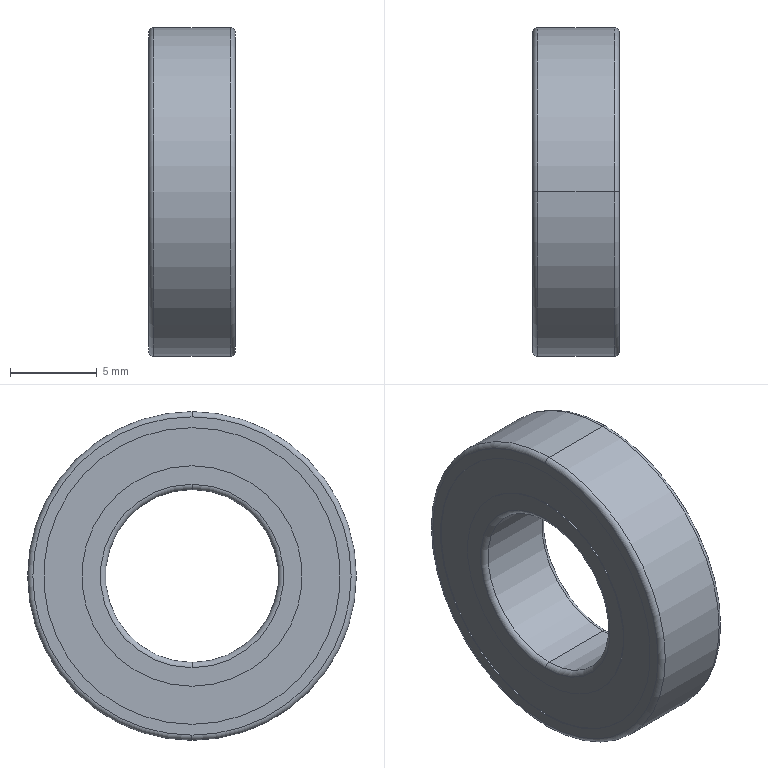Part | STEP file | 11-B6800ZZ11_B6800ZZ | 1 solid | 26 faces | box 5 x 19 x 19 mm | volume 1010 mm3 | cylinder 12 | torus 8 | plane 6 | commonest cylinder face diameters 12.74 x4 17.15 x4 10 x2 19 x2
STEP:
#1=CARTESIAN_POINT('',(4.7,0.,9.5));
#2=VERTEX_POINT('',#1);
#3=CARTESIAN_POINT('',(4.7,0.,-9.5));
#4=VERTEX_POINT('',#3);
#5=CARTESIAN_POINT('',(4.7,0.,0.));
#6=DIRECTION('',(-1.,0.,0.));
#7=DIRECTION('',(0.,0.,1.));
#8=AXIS2_PLACEMENT_3D('',#5,#6,#7);
#9=CIRCLE('',#8,9.5);
#10=EDGE_CURVE('',#2,#4,#9,.T.);
#11=ORIENTED_EDGE('',*,*,#10,.T.);
#12=CARTESIAN_POINT('',(0.3,0.,-9.5));
#13=VERTEX_POINT('',#12);
#14=CARTESIAN_POINT('',(5.,0.,-9.5));
#15=DIRECTION('',(-1.,0.,0.));
#16=VECTOR('',#15,1000.);
#17=LINE('',#14,#16);
#18=EDGE_CURVE('',#4,#13,#17,.T.);
#19=ORIENTED_EDGE('',*,*,#18,.T.);
#20=CARTESIAN_POINT('',(0.3,0.,9.5));
#21=VERTEX_POINT('',#20);
#22=CARTESIAN_POINT('',(0.3,0.,0.));
#23=DIRECTION('',(-1.,0.,0.));
#24=DIRECTION('',(0.,0.,1.));
#25=AXIS2_PLACEMENT_3D('',#22,#23,#24);
#26=CIRCLE('',#25,9.5);
#27=EDGE_CURVE('',#21,#13,#26,.T.);
#28=ORIENTED_EDGE('',*,*,#27,.F.);
#29=CARTESIAN_POINT('',(5.,0.,9.5));
#30=DIRECTION('',(-1.,0.,0.));
#31=VECTOR('',#30,1000.);
#32=LINE('',#29,#31);
#33=EDGE_CURVE('',#2,#21,#32,.T.);
#34=ORIENTED_EDGE('',*,*,#33,.F.);
#35=EDGE_LOOP('',(#11,#19,#28,#34));
#36=FACE_OUTER_BOUND('',#35,.T.);
#37=CARTESIAN_POINT('',(5.,0.,0.));
#38=DIRECTION('',(-1.,0.,0.));
#39=DIRECTION('',(0.,0.,1.));
#40=AXIS2_PLACEMENT_3D('',#37,#38,#39);
#41=CYLINDRICAL_SURFACE('',#40,9.5);
#42=ADVANCED_FACE('',(#36),#41,.T.);
#43=CARTESIAN_POINT('',(5.,0.,9.2));
#44=VERTEX_POINT('',#43);
#45=CARTESIAN_POINT('',(5.,0.,-9.2));
#46=VERTEX_POINT('',#45);
#47=CARTESIAN_POINT('',(5.,0.,0.));
#48=DIRECTION('',(-1.,0.,0.));
#49=DIRECTION('',(0.,0.,1.));
#50=AXIS2_PLACEMENT_3D('',#47,#48,#49);
#51=CIRCLE('',#50,9.2);
#52=EDGE_CURVE('',#44,#46,#51,.T.);
#53=ORIENTED_EDGE('',*,*,#52,.T.);
#54=CARTESIAN_POINT('',(4.7,0.,-9.2));
#55=DIRECTION('',(0.,1.,0.));
#56=DIRECTION('',(0.,0.,1.));
#57=AXIS2_PLACEMENT_3D('',#54,#55,#56);
#58=CIRCLE('',#57,0.3);
#59=EDGE_CURVE('',#46,#4,#58,.T.);
#60=ORIENTED_EDGE('',*,*,#59,.T.);
#61=ORIENTED_EDGE('',*,*,#10,.F.);
#62=CARTESIAN_POINT('',(4.7,0.,9.2));
#63=DIRECTION('',(0.,-1.,0.));
#64=DIRECTION('',(0.,0.,-1.));
#65=AXIS2_PLACEMENT_3D('',#62,#63,#64);
#66=CIRCLE('',#65,0.3);
#67=EDGE_CURVE('',#44,#2,#66,.T.);
#68=ORIENTED_EDGE('',*,*,#67,.F.);
#69=EDGE_LOOP('',(#53,#60,#61,#68));
#70=FACE_OUTER_BOUND('',#69,.T.);
#71=CARTESIAN_POINT('',(4.7,0.,0.));
#72=DIRECTION('',(-1.,0.,0.));
#73=DIRECTION('',(0.,0.,1.));
#74=AXIS2_PLACEMENT_3D('',#71,#72,#73);
#75=TOROIDAL_SURFACE('',#74,9.2,0.3);
#76=ADVANCED_FACE('',(#70),#75,.T.);
#77=CARTESIAN_POINT('',(5.,0.,-8.575));
#78=VERTEX_POINT('',#77);
#79=CARTESIAN_POINT('',(5.,0.,8.575));
#80=VERTEX_POINT('',#79);
#81=CARTESIAN_POINT('',(5.,0.,0.));
#82=DIRECTION('',(-1.,0.,0.));
#83=DIRECTION('',(0.,0.,1.));
#84=AXIS2_PLACEMENT_3D('',#81,#82,#83);
#85=CIRCLE('',#84,8.575);
#86=EDGE_CURVE('',#78,#80,#85,.T.);
#87=ORIENTED_EDGE('',*,*,#86,.F.);
#88=CARTESIAN_POINT('',(4.942,0.,-8.575));
#89=VERTEX_POINT('',#88);
#90=CARTESIAN_POINT('',(5.,0.,-8.575));
#91=DIRECTION('',(-1.,0.,0.));
#92=VECTOR('',#91,1000.);
#93=LINE('',#90,#92);
#94=EDGE_CURVE('',#78,#89,#93,.T.);
#95=ORIENTED_EDGE('',*,*,#94,.T.);
#96=CARTESIAN_POINT('',(4.942,0.,8.575));
#97=VERTEX_POINT('',#96);
#98=CARTESIAN_POINT('',(4.942,0.,0.));
#99=DIRECTION('',(-1.,0.,0.));
#100=DIRECTION('',(0.,0.,1.));
#101=AXIS2_PLACEMENT_3D('',#98,#99,#100);
#102=CIRCLE('',#101,8.575);
#103=EDGE_CURVE('',#89,#97,#102,.T.);
#104=ORIENTED_EDGE('',*,*,#103,.T.);
#105=CARTESIAN_POINT('',(5.,0.,8.575));
#106=DIRECTION('',(-1.,0.,0.));
#107=VECTOR('',#106,1000.);
#108=LINE('',#105,#107);
#109=EDGE_CURVE('',#80,#97,#108,.T.);
#110=ORIENTED_EDGE('',*,*,#109,.F.);
#111=EDGE_LOOP('',(#87,#95,#104,#110));
#112=FACE_OUTER_BOUND('',#111,.T.);
#113=CARTESIAN_POINT('',(5.,0.,0.));
#114=DIRECTION('',(-1.,0.,0.));
#115=DIRECTION('',(0.,0.,1.));
#116=AXIS2_PLACEMENT_3D('',#113,#114,#115);
#117=CYLINDRICAL_SURFACE('',#116,8.575);
#118=ADVANCED_FACE('',(#112),#117,.F.);
#119=CARTESIAN_POINT('',(5.,0.,6.37));
#120=VERTEX_POINT('',#119);
#121=CARTESIAN_POINT('',(5.,0.,-6.37));
#122=VERTEX_POINT('',#121);
#123=CARTESIAN_POINT('',(5.,0.,0.));
#124=DIRECTION('',(-1.,0.,0.));
#125=DIRECTION('',(0.,0.,1.));
#126=AXIS2_PLACEMENT_3D('',#123,#124,#125);
#127=CIRCLE('',#126,6.37);
#128=EDGE_CURVE('',#120,#122,#127,.T.);
#129=ORIENTED_EDGE('',*,*,#128,.T.);
#130=CARTESIAN_POINT('',(4.942,0.,-6.37));
#131=VERTEX_POINT('',#130);
#132=CARTESIAN_POINT('',(5.,0.,-6.37));
#133=DIRECTION('',(-1.,0.,0.));
#134=VECTOR('',#133,1000.);
#135=LINE('',#132,#134);
#136=EDGE_CURVE('',#122,#131,#135,.T.);
#137=ORIENTED_EDGE('',*,*,#136,.T.);
#138=CARTESIAN_POINT('',(4.942,0.,6.37));
#139=VERTEX_POINT('',#138);
#140=CARTESIAN_POINT('',(4.942,0.,0.));
#141=DIRECTION('',(-1.,0.,0.));
#142=DIRECTION('',(0.,0.,1.));
#143=AXIS2_PLACEMENT_3D('',#140,#141,#142);
#144=CIRCLE('',#143,6.37);
#145=EDGE_CURVE('',#139,#131,#144,.T.);
#146=ORIENTED_EDGE('',*,*,#145,.F.);
#147=CARTESIAN_POINT('',(5.,0.,6.37));
#148=DIRECTION('',(-1.,0.,0.));
#149=VECTOR('',#148,1000.);
#150=LINE('',#147,#149);
#151=EDGE_CURVE('',#120,#139,#150,.T.);
#152=ORIENTED_EDGE('',*,*,#151,.F.);
#153=EDGE_LOOP('',(#129,#137,#146,#152));
#154=FACE_OUTER_BOUND('',#153,.T.);
#155=CARTESIAN_POINT('',(5.,0.,0.));
#156=DIRECTION('',(-1.,0.,0.));
#157=DIRECTION('',(0.,0.,1.));
#158=AXIS2_PLACEMENT_3D('',#155,#156,#157);
#159=CYLINDRICAL_SURFACE('',#158,6.37);
#160=ADVANCED_FACE('',(#154),#159,.T.);
#161=CARTESIAN_POINT('',(4.7,0.,5.));
#162=VERTEX_POINT('',#161);
#163=CARTESIAN_POINT('',(4.7,0.,-5.));
#164=VERTEX_POINT('',#163);
#165=CARTESIAN_POINT('',(4.7,0.,0.));
#166=DIRECTION('',(-1.,0.,0.));
#167=DIRECTION('',(0.,0.,1.));
#168=AXIS2_PLACEMENT_3D('',#165,#166,#167);
#169=CIRCLE('',#168,5.);
#170=EDGE_CURVE('',#162,#164,#169,.T.);
#171=ORIENTED_EDGE('',*,*,#170,.T.);
#172=CARTESIAN_POINT('',(5.,0.,-5.3));
#173=VERTEX_POINT('',#172);
#174=CARTESIAN_POINT('',(4.7,0.,-5.3));
#175=DIRECTION('',(0.,1.,0.));
#176=DIRECTION('',(0.,0.,1.));
#177=AXIS2_PLACEMENT_3D('',#174,#175,#176);
#178=CIRCLE('',#177,0.3);
#179=EDGE_CURVE('',#164,#173,#178,.T.);
#180=ORIENTED_EDGE('',*,*,#179,.T.);
#181=CARTESIAN_POINT('',(5.,0.,5.3));
#182=VERTEX_POINT('',#181);
#183=CARTESIAN_POINT('',(5.,0.,0.));
#184=DIRECTION('',(-1.,0.,0.));
#185=DIRECTION('',(0.,0.,1.));
#186=AXIS2_PLACEMENT_3D('',#183,#184,#185);
#187=CIRCLE('',#186,5.3);
#188=EDGE_CURVE('',#182,#173,#187,.T.);
#189=ORIENTED_EDGE('',*,*,#188,.F.);
#190=CARTESIAN_POINT('',(4.7,0.,5.3));
#191=DIRECTION('',(0.,-1.,0.));
#192=DIRECTION('',(0.,0.,-1.));
#193=AXIS2_PLACEMENT_3D('',#190,#191,#192);
#194=CIRCLE('',#193,0.3);
#195=EDGE_CURVE('',#162,#182,#194,.T.);
#196=ORIENTED_EDGE('',*,*,#195,.F.);
#197=EDGE_LOOP('',(#171,#180,#189,#196));
#198=FACE_OUTER_BOUND('',#197,.T.);
#199=CARTESIAN_POINT('',(4.7,0.,0.));
#200=DIRECTION('',(-1.,0.,0.));
#201=DIRECTION('',(0.,0.,1.));
#202=AXIS2_PLACEMENT_3D('',#199,#200,#201);
#203=TOROIDAL_SURFACE('',#202,5.3,0.3);
#204=ADVANCED_FACE('',(#198),#203,.T.);
#205=CARTESIAN_POINT('',(4.7,0.,0.));
#206=DIRECTION('',(-1.,0.,0.));
#207=DIRECTION('',(0.,0.,1.));
#208=AXIS2_PLACEMENT_3D('',#205,#206,#207);
#209=CIRCLE('',#208,5.);
#210=EDGE_CURVE('',#164,#162,#209,.T.);
#211=ORIENTED_EDGE('',*,*,#210,.F.);
#212=CARTESIAN_POINT('',(0.3,0.,-5.));
#213=VERTEX_POINT('',#212);
#214=CARTESIAN_POINT('',(5.,0.,-5.));
#215=DIRECTION('',(-1.,0.,0.));
#216=VECTOR('',#215,1000.);
#217=LINE('',#214,#216);
#218=EDGE_CURVE('',#164,#213,#217,.T.);
#219=ORIENTED_EDGE('',*,*,#218,.T.);
#220=CARTESIAN_POINT('',(0.3,0.,5.));
#221=VERTEX_POINT('',#220);
#222=CARTESIAN_POINT('',(0.3,0.,0.));
#223=DIRECTION('',(-1.,0.,0.));
#224=DIRECTION('',(0.,0.,1.));
#225=AXIS2_PLACEMENT_3D('',#222,#223,#224);
#226=CIRCLE('',#225,5.);
#227=EDGE_CURVE('',#213,#221,#226,.T.);
#228=ORIENTED_EDGE('',*,*,#227,.T.);
#229=CARTESIAN_POINT('',(5.,0.,5.));
#230=DIRECTION('',(-1.,0.,0.));
#231=VECTOR('',#230,1000.);
#232=LINE('',#229,#231);
#233=EDGE_CURVE('',#162,#221,#232,.T.);
#234=ORIENTED_EDGE('',*,*,#233,.F.);
#235=EDGE_LOOP('',(#211,#219,#228,#234));
#236=FACE_OUTER_BOUND('',#235,.T.);
#237=CARTESIAN_POINT('',(5.,0.,0.));
#238=DIRECTION('',(-1.,0.,0.));
#239=DIRECTION('',(0.,0.,1.));
#240=AXIS2_PLACEMENT_3D('',#237,#238,#239);
#241=CYLINDRICAL_SURFACE('',#240,5.);
#242=ADVANCED_FACE('',(#236),#241,.F.);
#243=CARTESIAN_POINT('',(0.,0.,5.3));
#244=VERTEX_POINT('',#243);
#245=CARTESIAN_POINT('',(0.,0.,-5.3));
#246=VERTEX_POINT('',#245);
#247=CARTESIAN_POINT('',(0.,0.,0.));
#248=DIRECTION('',(-1.,0.,0.));
#249=DIRECTION('',(0.,0.,1.));
#250=AXIS2_PLACEMENT_3D('',#247,#248,#249);
#251=CIRCLE('',#250,5.3);
#252=EDGE_CURVE('',#244,#246,#251,.T.);
#253=ORIENTED_EDGE('',*,*,#252,.T.);
#254=CARTESIAN_POINT('',(0.3,0.,-5.3));
#255=DIRECTION('',(0.,1.,0.));
#256=DIRECTION('',(0.,0.,1.));
#257=AXIS2_PLACEMENT_3D('',#254,#255,#256);
#258=CIRCLE('',#257,0.3);
#259=EDGE_CURVE('',#246,#213,#258,.T.);
#260=ORIENTED_EDGE('',*,*,#259,.T.);
#261=CARTESIAN_POINT('',(0.3,0.,0.));
#262=DIRECTION('',(-1.,0.,0.));
#263=DIRECTION('',(0.,0.,1.));
#264=AXIS2_PLACEMENT_3D('',#261,#262,#263);
#265=CIRCLE('',#264,5.);
#266=EDGE_CURVE('',#221,#213,#265,.T.);
#267=ORIENTED_EDGE('',*,*,#266,.F.);
#268=CARTESIAN_POINT('',(0.3,0.,5.3));
#269=DIRECTION('',(0.,-1.,0.));
#270=DIRECTION('',(0.,0.,-1.));
#271=AXIS2_PLACEMENT_3D('',#268,#269,#270);
#272=CIRCLE('',#271,0.3);
#273=EDGE_CURVE('',#244,#221,#272,.T.);
#274=ORIENTED_EDGE('',*,*,#273,.F.);
#275=EDGE_LOOP('',(#253,#260,#267,#274));
#276=FACE_OUTER_BOUND('',#275,.T.);
#277=CARTESIAN_POINT('',(0.3,0.,0.));
#278=DIRECTION('',(-1.,0.,0.));
#279=DIRECTION('',(0.,0.,1.));
#280=AXIS2_PLACEMENT_3D('',#277,#278,#279);
#281=TOROIDAL_SURFACE('',#280,5.3,0.3);
#282=ADVANCED_FACE('',(#276),#281,.T.);
#283=CARTESIAN_POINT('',(0.0575,0.,6.37));
#284=VERTEX_POINT('',#283);
#285=CARTESIAN_POINT('',(0.0575,0.,-6.37));
#286=VERTEX_POINT('',#285);
#287=CARTESIAN_POINT('',(0.0575,0.,0.));
#288=DIRECTION('',(-1.,0.,0.));
#289=DIRECTION('',(0.,0.,1.));
#290=AXIS2_PLACEMENT_3D('',#287,#288,#289);
#291=CIRCLE('',#290,6.37);
#292=EDGE_CURVE('',#284,#286,#291,.T.);
#293=ORIENTED_EDGE('',*,*,#292,.T.);
#294=CARTESIAN_POINT('',(0.,0.,-6.37));
#295=VERTEX_POINT('',#294);
#296=CARTESIAN_POINT('',(5.,0.,-6.37));
#297=DIRECTION('',(-1.,0.,0.));
#298=VECTOR('',#297,1000.);
#299=LINE('',#296,#298);
#300=EDGE_CURVE('',#286,#295,#299,.T.);
#301=ORIENTED_EDGE('',*,*,#300,.T.);
#302=CARTESIAN_POINT('',(0.,0.,6.37));
#303=VERTEX_POINT('',#302);
#304=CARTESIAN_POINT('',(0.,0.,0.));
#305=DIRECTION('',(-1.,0.,0.));
#306=DIRECTION('',(0.,0.,1.));
#307=AXIS2_PLACEMENT_3D('',#304,#305,#306);
#308=CIRCLE('',#307,6.37);
#309=EDGE_CURVE('',#303,#295,#308,.T.);
#310=ORIENTED_EDGE('',*,*,#309,.F.);
#311=CARTESIAN_POINT('',(5.,0.,6.37));
#312=DIRECTION('',(-1.,0.,0.));
#313=VECTOR('',#312,1000.);
#314=LINE('',#311,#313);
#315=EDGE_CURVE('',#284,#303,#314,.T.);
#316=ORIENTED_EDGE('',*,*,#315,.F.);
#317=EDGE_LOOP('',(#293,#301,#310,#316));
#318=FACE_OUTER_BOUND('',#317,.T.);
#319=CARTESIAN_POINT('',(5.,0.,0.));
#320=DIRECTION('',(-1.,0.,0.));
#321=DIRECTION('',(0.,0.,1.));
#322=AXIS2_PLACEMENT_3D('',#319,#320,#321);
#323=CYLINDRICAL_SURFACE('',#322,6.37);
#324=ADVANCED_FACE('',(#318),#323,.T.);
#325=CARTESIAN_POINT('',(0.0575,0.,-8.575));
#326=VERTEX_POINT('',#325);
#327=CARTESIAN_POINT('',(0.0575,0.,8.575));
#328=VERTEX_POINT('',#327);
#329=CARTESIAN_POINT('',(0.0575,0.,0.));
#330=DIRECTION('',(-1.,0.,0.));
#331=DIRECTION('',(0.,0.,1.));
#332=AXIS2_PLACEMENT_3D('',#329,#330,#331);
#333=CIRCLE('',#332,8.575);
#334=EDGE_CURVE('',#326,#328,#333,.T.);
#335=ORIENTED_EDGE('',*,*,#334,.F.);
#336=CARTESIAN_POINT('',(0.,0.,-8.575));
#337=VERTEX_POINT('',#336);
#338=CARTESIAN_POINT('',(5.,0.,-8.575));
#339=DIRECTION('',(-1.,0.,0.));
#340=VECTOR('',#339,1000.);
#341=LINE('',#338,#340);
#342=EDGE_CURVE('',#326,#337,#341,.T.);
#343=ORIENTED_EDGE('',*,*,#342,.T.);
#344=CARTESIAN_POINT('',(0.,0.,8.575));
#345=VERTEX_POINT('',#344);
#346=CARTESIAN_POINT('',(0.,0.,0.));
#347=DIRECTION('',(-1.,0.,0.));
#348=DIRECTION('',(0.,0.,1.));
#349=AXIS2_PLACEMENT_3D('',#346,#347,#348);
#350=CIRCLE('',#349,8.575);
#351=EDGE_CURVE('',#337,#345,#350,.T.);
#352=ORIENTED_EDGE('',*,*,#351,.T.);
#353=CARTESIAN_POINT('',(5.,0.,8.575));
#354=DIRECTION('',(-1.,0.,0.));
#355=VECTOR('',#354,1000.);
#356=LINE('',#353,#355);
#357=EDGE_CURVE('',#328,#345,#356,.T.);
#358=ORIENTED_EDGE('',*,*,#357,.F.);
#359=EDGE_LOOP('',(#335,#343,#352,#358));
#360=FACE_OUTER_BOUND('',#359,.T.);
#361=CARTESIAN_POINT('',(5.,0.,0.));
#362=DIRECTION('',(-1.,0.,0.));
#363=DIRECTION('',(0.,0.,1.));
#364=AXIS2_PLACEMENT_3D('',#361,#362,#363);
#365=CYLINDRICAL_SURFACE('',#364,8.575);
#366=ADVANCED_FACE('',(#360),#365,.F.);
#367=ORIENTED_EDGE('',*,*,#27,.T.);
#368=CARTESIAN_POINT('',(0.,0.,-9.2));
#369=VERTEX_POINT('',#368);
#370=CARTESIAN_POINT('',(0.3,0.,-9.2));
#371=DIRECTION('',(0.,1.,0.));
#372=DIRECTION('',(0.,0.,1.));
#373=AXIS2_PLACEMENT_3D('',#370,#371,#372);
#374=CIRCLE('',#373,0.3);
#375=EDGE_CURVE('',#13,#369,#374,.T.);
#376=ORIENTED_EDGE('',*,*,#375,.T.);
#377=CARTESIAN_POINT('',(0.,0.,9.2));
#378=VERTEX_POINT('',#377);
#379=CARTESIAN_POINT('',(0.,0.,0.));
#380=DIRECTION('',(-1.,0.,0.));
#381=DIRECTION('',(0.,0.,1.));
#382=AXIS2_PLACEMENT_3D('',#379,#380,#381);
#383=CIRCLE('',#382,9.2);
#384=EDGE_CURVE('',#378,#369,#383,.T.);
#385=ORIENTED_EDGE('',*,*,#384,.F.);
#386=CARTESIAN_POINT('',(0.3,0.,9.2));
#387=DIRECTION('',(0.,-1.,0.));
#388=DIRECTION('',(0.,0.,-1.));
#389=AXIS2_PLACEMENT_3D('',#386,#387,#388);
#390=CIRCLE('',#389,0.3);
#391=EDGE_CURVE('',#21,#378,#390,.T.);
#392=ORIENTED_EDGE('',*,*,#391,.F.);
#393=EDGE_LOOP('',(#367,#376,#385,#392));
#394=FACE_OUTER_BOUND('',#393,.T.);
#395=CARTESIAN_POINT('',(0.3,0.,0.));
#396=DIRECTION('',(-1.,0.,0.));
#397=DIRECTION('',(0.,0.,1.));
#398=AXIS2_PLACEMENT_3D('',#395,#396,#397);
#399=TOROIDAL_SURFACE('',#398,9.2,0.3);
#400=ADVANCED_FACE('',(#394),#399,.T.);
#401=ORIENTED_EDGE('',*,*,#375,.F.);
#402=CARTESIAN_POINT('',(0.3,0.,0.));
#403=DIRECTION('',(-1.,0.,0.));
#404=DIRECTION('',(0.,0.,1.));
#405=AXIS2_PLACEMENT_3D('',#402,#403,#404);
#406=CIRCLE('',#405,9.5);
#407=EDGE_CURVE('',#13,#21,#406,.T.);
#408=ORIENTED_EDGE('',*,*,#407,.T.);
#409=ORIENTED_EDGE('',*,*,#391,.T.);
#410=CARTESIAN_POINT('',(0.,0.,0.));
#411=DIRECTION('',(-1.,0.,0.));
#412=DIRECTION('',(0.,0.,1.));
#413=AXIS2_PLACEMENT_3D('',#410,#411,#412);
#414=CIRCLE('',#413,9.2);
#415=EDGE_CURVE('',#369,#378,#414,.T.);
#416=ORIENTED_EDGE('',*,*,#415,.F.);
#417=EDGE_LOOP('',(#401,#408,#409,#416));
#418=FACE_OUTER_BOUND('',#417,.T.);
#419=CARTESIAN_POINT('',(0.3,0.,0.));
#420=DIRECTION('',(-1.,0.,0.));
#421=DIRECTION('',(0.,0.,1.));
#422=AXIS2_PLACEMENT_3D('',#419,#420,#421);
#423=TOROIDAL_SURFACE('',#422,9.2,0.3);
#424=ADVANCED_FACE('',(#418),#423,.T.);
#425=CARTESIAN_POINT('',(0.,0.,0.));
#426=DIRECTION('',(-1.,0.,0.));
#427=DIRECTION('',(0.,0.,1.));
#428=AXIS2_PLACEMENT_3D('',#425,#426,#427);
#429=CIRCLE('',#428,8.575);
#430=EDGE_CURVE('',#345,#337,#429,.T.);
#431=ORIENTED_EDGE('',*,*,#430,.F.);
#432=ORIENTED_EDGE('',*,*,#351,.F.);
#433=EDGE_LOOP('',(#431,#432));
#434=FACE_BOUND('',#433,.T.);
#435=ORIENTED_EDGE('',*,*,#384,.T.);
#436=ORIENTED_EDGE('',*,*,#415,.T.);
#437=EDGE_LOOP('',(#435,#436));
#438=FACE_OUTER_BOUND('',#437,.T.);
#439=CARTESIAN_POINT('',(0.,9.2,0.));
#440=DIRECTION('',(1.,0.,0.));
#441=DIRECTION('',(0.,0.,-1.));
#442=AXIS2_PLACEMENT_3D('',#439,#440,#441);
#443=PLANE('',#442);
#444=ADVANCED_FACE('',(#434,#438),#443,.F.);
#445=ORIENTED_EDGE('',*,*,#342,.F.);
#446=CARTESIAN_POINT('',(0.0575,0.,0.));
#447=DIRECTION('',(-1.,0.,0.));
#448=DIRECTION('',(0.,0.,1.));
#449=AXIS2_PLACEMENT_3D('',#446,#447,#448);
#450=CIRCLE('',#449,8.575);
#451=EDGE_CURVE('',#328,#326,#450,.T.);
#452=ORIENTED_EDGE('',*,*,#451,.F.);
#453=ORIENTED_EDGE('',*,*,#357,.T.);
#454=ORIENTED_EDGE('',*,*,#430,.T.);
#455=EDGE_LOOP('',(#445,#452,#453,#454));
#456=FACE_OUTER_BOUND('',#455,.T.);
#457=CARTESIAN_POINT('',(5.,0.,0.));
#458=DIRECTION('',(-1.,0.,0.));
#459=DIRECTION('',(0.,0.,1.));
#460=AXIS2_PLACEMENT_3D('',#457,#458,#459);
#461=CYLINDRICAL_SURFACE('',#460,8.575);
#462=ADVANCED_FACE('',(#456),#461,.F.);
#463=ORIENTED_EDGE('',*,*,#292,.F.);
#464=CARTESIAN_POINT('',(0.0575,0.,0.));
#465=DIRECTION('',(-1.,0.,0.));
#466=DIRECTION('',(0.,0.,1.));
#467=AXIS2_PLACEMENT_3D('',#464,#465,#466);
#468=CIRCLE('',#467,6.37);
#469=EDGE_CURVE('',#286,#284,#468,.T.);
#470=ORIENTED_EDGE('',*,*,#469,.F.);
#471=EDGE_LOOP('',(#463,#470));
#472=FACE_BOUND('',#471,.T.);
#473=ORIENTED_EDGE('',*,*,#451,.T.);
#474=ORIENTED_EDGE('',*,*,#334,.T.);
#475=EDGE_LOOP('',(#473,#474));
#476=FACE_OUTER_BOUND('',#475,.T.);
#477=CARTESIAN_POINT('',(0.0575,8.575,0.));
#478=DIRECTION('',(1.,0.,0.));
#479=DIRECTION('',(0.,0.,-1.));
#480=AXIS2_PLACEMENT_3D('',#477,#478,#479);
#481=PLANE('',#480);
#482=ADVANCED_FACE('',(#472,#476),#481,.F.);
#483=ORIENTED_EDGE('',*,*,#300,.F.);
#484=ORIENTED_EDGE('',*,*,#469,.T.);
#485=ORIENTED_EDGE('',*,*,#315,.T.);
#486=CARTESIAN_POINT('',(0.,0.,0.));
#487=DIRECTION('',(-1.,0.,0.));
#488=DIRECTION('',(0.,0.,1.));
#489=AXIS2_PLACEMENT_3D('',#486,#487,#488);
#490=CIRCLE('',#489,6.37);
#491=EDGE_CURVE('',#295,#303,#490,.T.);
#492=ORIENTED_EDGE('',*,*,#491,.F.);
#493=EDGE_LOOP('',(#483,#484,#485,#492));
#494=FACE_OUTER_BOUND('',#493,.T.);
#495=CARTESIAN_POINT('',(5.,0.,0.));
#496=DIRECTION('',(-1.,0.,0.));
#497=DIRECTION('',(0.,0.,1.));
#498=AXIS2_PLACEMENT_3D('',#495,#496,#497);
#499=CYLINDRICAL_SURFACE('',#498,6.37);
#500=ADVANCED_FACE('',(#494),#499,.T.);
#501=ORIENTED_EDGE('',*,*,#252,.F.);
#502=CARTESIAN_POINT('',(0.,0.,0.));
#503=DIRECTION('',(-1.,0.,0.));
#504=DIRECTION('',(0.,0.,1.));
#505=AXIS2_PLACEMENT_3D('',#502,#503,#504);
#506=CIRCLE('',#505,5.3);
#507=EDGE_CURVE('',#246,#244,#506,.T.);
#508=ORIENTED_EDGE('',*,*,#507,.F.);
#509=EDGE_LOOP('',(#501,#508));
#510=FACE_BOUND('',#509,.T.);
#511=ORIENTED_EDGE('',*,*,#309,.T.);
#512=ORIENTED_EDGE('',*,*,#491,.T.);
#513=EDGE_LOOP('',(#511,#512));
#514=FACE_OUTER_BOUND('',#513,.T.);
#515=CARTESIAN_POINT('',(0.,6.37,0.));
#516=DIRECTION('',(1.,0.,0.));
#517=DIRECTION('',(0.,0.,-1.));
#518=AXIS2_PLACEMENT_3D('',#515,#516,#517);
#519=PLANE('',#518);
#520=ADVANCED_FACE('',(#510,#514),#519,.F.);
#521=ORIENTED_EDGE('',*,*,#259,.F.);
#522=ORIENTED_EDGE('',*,*,#507,.T.);
#523=ORIENTED_EDGE('',*,*,#273,.T.);
#524=ORIENTED_EDGE('',*,*,#227,.F.);
#525=EDGE_LOOP('',(#521,#522,#523,#524));
#526=FACE_OUTER_BOUND('',#525,.T.);
#527=CARTESIAN_POINT('',(0.3,0.,0.));
#528=DIRECTION('',(-1.,0.,0.));
#529=DIRECTION('',(0.,0.,1.));
#530=AXIS2_PLACEMENT_3D('',#527,#528,#529);
#531=TOROIDAL_SURFACE('',#530,5.3,0.3);
#532=ADVANCED_FACE('',(#526),#531,.T.);
#533=ORIENTED_EDGE('',*,*,#218,.F.);
#534=ORIENTED_EDGE('',*,*,#170,.F.);
#535=ORIENTED_EDGE('',*,*,#233,.T.);
#536=ORIENTED_EDGE('',*,*,#266,.T.);
#537=EDGE_LOOP('',(#533,#534,#535,#536));
#538=FACE_OUTER_BOUND('',#537,.T.);
#539=CARTESIAN_POINT('',(5.,0.,0.));
#540=DIRECTION('',(-1.,0.,0.));
#541=DIRECTION('',(0.,0.,1.));
#542=AXIS2_PLACEMENT_3D('',#539,#540,#541);
#543=CYLINDRICAL_SURFACE('',#542,5.);
#544=ADVANCED_FACE('',(#538),#543,.F.);
#545=ORIENTED_EDGE('',*,*,#179,.F.);
#546=ORIENTED_EDGE('',*,*,#210,.T.);
#547=ORIENTED_EDGE('',*,*,#195,.T.);
#548=CARTESIAN_POINT('',(5.,0.,0.));
#549=DIRECTION('',(-1.,0.,0.));
#550=DIRECTION('',(0.,0.,1.));
#551=AXIS2_PLACEMENT_3D('',#548,#549,#550);
#552=CIRCLE('',#551,5.3);
#553=EDGE_CURVE('',#173,#182,#552,.T.);
#554=ORIENTED_EDGE('',*,*,#553,.F.);
#555=EDGE_LOOP('',(#545,#546,#547,#554));
#556=FACE_OUTER_BOUND('',#555,.T.);
#557=CARTESIAN_POINT('',(4.7,0.,0.));
#558=DIRECTION('',(-1.,0.,0.));
#559=DIRECTION('',(0.,0.,1.));
#560=AXIS2_PLACEMENT_3D('',#557,#558,#559);
#561=TOROIDAL_SURFACE('',#560,5.3,0.3);
#562=ADVANCED_FACE('',(#556),#561,.T.);
#563=ORIENTED_EDGE('',*,*,#128,.F.);
#564=CARTESIAN_POINT('',(5.,0.,0.));
#565=DIRECTION('',(-1.,0.,0.));
#566=DIRECTION('',(0.,0.,1.));
#567=AXIS2_PLACEMENT_3D('',#564,#565,#566);
#568=CIRCLE('',#567,6.37);
#569=EDGE_CURVE('',#122,#120,#568,.T.);
#570=ORIENTED_EDGE('',*,*,#569,.F.);
#571=EDGE_LOOP('',(#563,#570));
#572=FACE_OUTER_BOUND('',#571,.T.);
#573=ORIENTED_EDGE('',*,*,#188,.T.);
#574=ORIENTED_EDGE('',*,*,#553,.T.);
#575=EDGE_LOOP('',(#573,#574));
#576=FACE_BOUND('',#575,.T.);
#577=CARTESIAN_POINT('',(5.,5.3,0.));
#578=DIRECTION('',(-1.,0.,0.));
#579=DIRECTION('',(0.,0.,1.));
#580=AXIS2_PLACEMENT_3D('',#577,#578,#579);
#581=PLANE('',#580);
#582=ADVANCED_FACE('',(#572,#576),#581,.F.);
#583=ORIENTED_EDGE('',*,*,#136,.F.);
#584=ORIENTED_EDGE('',*,*,#569,.T.);
#585=ORIENTED_EDGE('',*,*,#151,.T.);
#586=CARTESIAN_POINT('',(4.942,0.,0.));
#587=DIRECTION('',(-1.,0.,0.));
#588=DIRECTION('',(0.,0.,1.));
#589=AXIS2_PLACEMENT_3D('',#586,#587,#588);
#590=CIRCLE('',#589,6.37);
#591=EDGE_CURVE('',#131,#139,#590,.T.);
#592=ORIENTED_EDGE('',*,*,#591,.F.);
#593=EDGE_LOOP('',(#583,#584,#585,#592));
#594=FACE_OUTER_BOUND('',#593,.T.);
#595=CARTESIAN_POINT('',(5.,0.,0.));
#596=DIRECTION('',(-1.,0.,0.));
#597=DIRECTION('',(0.,0.,1.));
#598=AXIS2_PLACEMENT_3D('',#595,#596,#597);
#599=CYLINDRICAL_SURFACE('',#598,6.37);
#600=ADVANCED_FACE('',(#594),#599,.T.);
#601=CARTESIAN_POINT('',(4.942,0.,0.));
#602=DIRECTION('',(-1.,0.,0.));
#603=DIRECTION('',(0.,0.,1.));
#604=AXIS2_PLACEMENT_3D('',#601,#602,#603);
#605=CIRCLE('',#604,8.575);
#606=EDGE_CURVE('',#97,#89,#605,.T.);
#607=ORIENTED_EDGE('',*,*,#606,.F.);
#608=ORIENTED_EDGE('',*,*,#103,.F.);
#609=EDGE_LOOP('',(#607,#608));
#610=FACE_OUTER_BOUND('',#609,.T.);
#611=ORIENTED_EDGE('',*,*,#145,.T.);
#612=ORIENTED_EDGE('',*,*,#591,.T.);
#613=EDGE_LOOP('',(#611,#612));
#614=FACE_BOUND('',#613,.T.);
#615=CARTESIAN_POINT('',(4.942,6.37,0.));
#616=DIRECTION('',(-1.,0.,0.));
#617=DIRECTION('',(0.,0.,1.));
#618=AXIS2_PLACEMENT_3D('',#615,#616,#617);
#619=PLANE('',#618);
#620=ADVANCED_FACE('',(#610,#614),#619,.F.);
#621=ORIENTED_EDGE('',*,*,#94,.F.);
#622=CARTESIAN_POINT('',(5.,0.,0.));
#623=DIRECTION('',(-1.,0.,0.));
#624=DIRECTION('',(0.,0.,1.));
#625=AXIS2_PLACEMENT_3D('',#622,#623,#624);
#626=CIRCLE('',#625,8.575);
#627=EDGE_CURVE('',#80,#78,#626,.T.);
#628=ORIENTED_EDGE('',*,*,#627,.F.);
#629=ORIENTED_EDGE('',*,*,#109,.T.);
#630=ORIENTED_EDGE('',*,*,#606,.T.);
#631=EDGE_LOOP('',(#621,#628,#629,#630));
#632=FACE_OUTER_BOUND('',#631,.T.);
#633=CARTESIAN_POINT('',(5.,0.,0.));
#634=DIRECTION('',(-1.,0.,0.));
#635=DIRECTION('',(0.,0.,1.));
#636=AXIS2_PLACEMENT_3D('',#633,#634,#635);
#637=CYLINDRICAL_SURFACE('',#636,8.575);
#638=ADVANCED_FACE('',(#632),#637,.F.);
#639=ORIENTED_EDGE('',*,*,#52,.F.);
#640=CARTESIAN_POINT('',(5.,0.,0.));
#641=DIRECTION('',(-1.,0.,0.));
#642=DIRECTION('',(0.,0.,1.));
#643=AXIS2_PLACEMENT_3D('',#640,#641,#642);
#644=CIRCLE('',#643,9.2);
#645=EDGE_CURVE('',#46,#44,#644,.T.);
#646=ORIENTED_EDGE('',*,*,#645,.F.);
#647=EDGE_LOOP('',(#639,#646));
#648=FACE_OUTER_BOUND('',#647,.T.);
#649=ORIENTED_EDGE('',*,*,#627,.T.);
#650=ORIENTED_EDGE('',*,*,#86,.T.);
#651=EDGE_LOOP('',(#649,#650));
#652=FACE_BOUND('',#651,.T.);
#653=CARTESIAN_POINT('',(5.,8.575,0.));
#654=DIRECTION('',(-1.,0.,0.));
#655=DIRECTION('',(0.,0.,1.));
#656=AXIS2_PLACEMENT_3D('',#653,#654,#655);
#657=PLANE('',#656);
#658=ADVANCED_FACE('',(#648,#652),#657,.F.);
#659=ORIENTED_EDGE('',*,*,#59,.F.);
#660=ORIENTED_EDGE('',*,*,#645,.T.);
#661=ORIENTED_EDGE('',*,*,#67,.T.);
#662=CARTESIAN_POINT('',(4.7,0.,0.));
#663=DIRECTION('',(-1.,0.,0.));
#664=DIRECTION('',(0.,0.,1.));
#665=AXIS2_PLACEMENT_3D('',#662,#663,#664);
#666=CIRCLE('',#665,9.5);
#667=EDGE_CURVE('',#4,#2,#666,.T.);
#668=ORIENTED_EDGE('',*,*,#667,.F.);
#669=EDGE_LOOP('',(#659,#660,#661,#668));
#670=FACE_OUTER_BOUND('',#669,.T.);
#671=CARTESIAN_POINT('',(4.7,0.,0.));
#672=DIRECTION('',(-1.,0.,0.));
#673=DIRECTION('',(0.,0.,1.));
#674=AXIS2_PLACEMENT_3D('',#671,#672,#673);
#675=TOROIDAL_SURFACE('',#674,9.2,0.3);
#676=ADVANCED_FACE('',(#670),#675,.T.);
#677=ORIENTED_EDGE('',*,*,#18,.F.);
#678=ORIENTED_EDGE('',*,*,#667,.T.);
#679=ORIENTED_EDGE('',*,*,#33,.T.);
#680=ORIENTED_EDGE('',*,*,#407,.F.);
#681=EDGE_LOOP('',(#677,#678,#679,#680));
#682=FACE_OUTER_BOUND('',#681,.T.);
#683=CARTESIAN_POINT('',(5.,0.,0.));
#684=DIRECTION('',(-1.,0.,0.));
#685=DIRECTION('',(0.,0.,1.));
#686=AXIS2_PLACEMENT_3D('',#683,#684,#685);
#687=CYLINDRICAL_SURFACE('',#686,9.5);
#688=ADVANCED_FACE('',(#682),#687,.T.);
#689=CLOSED_SHELL('',(#42,#76,#118,#160,#204,#242,#282,#324,#366,#400,#424,#444,#462,#482,#500,#520,#532,#544,#562,#582,#600,#620,#638,#658,#676,#688));
#690=MANIFOLD_SOLID_BREP('',#689);
#691=CARTESIAN_POINT('',(0.,0.,0.));
#692=DIRECTION('',(0.,0.,1.));
#693=DIRECTION('',(1.,0.,0.));
#694=AXIS2_PLACEMENT_3D('',#691,#692,#693);
#695=(LENGTH_UNIT()NAMED_UNIT(*)SI_UNIT(.MILLI.,.METRE.));
#696=UNCERTAINTY_MEASURE_WITH_UNIT(LENGTH_MEASURE(0.00001),#695,'','');
#697=(NAMED_UNIT(*)PLANE_ANGLE_UNIT()SI_UNIT($,.RADIAN.));
#698=(NAMED_UNIT(*)SI_UNIT($,.STERADIAN.)SOLID_ANGLE_UNIT());
#699=(GEOMETRIC_REPRESENTATION_CONTEXT(3)GLOBAL_UNCERTAINTY_ASSIGNED_CONTEXT((#696))GLOBAL_UNIT_ASSIGNED_CONTEXT((#695,#697,#698))REPRESENTATION_CONTEXT('',''));
#700=ADVANCED_BREP_SHAPE_REPRESENTATION('',(#690,#694),#699);